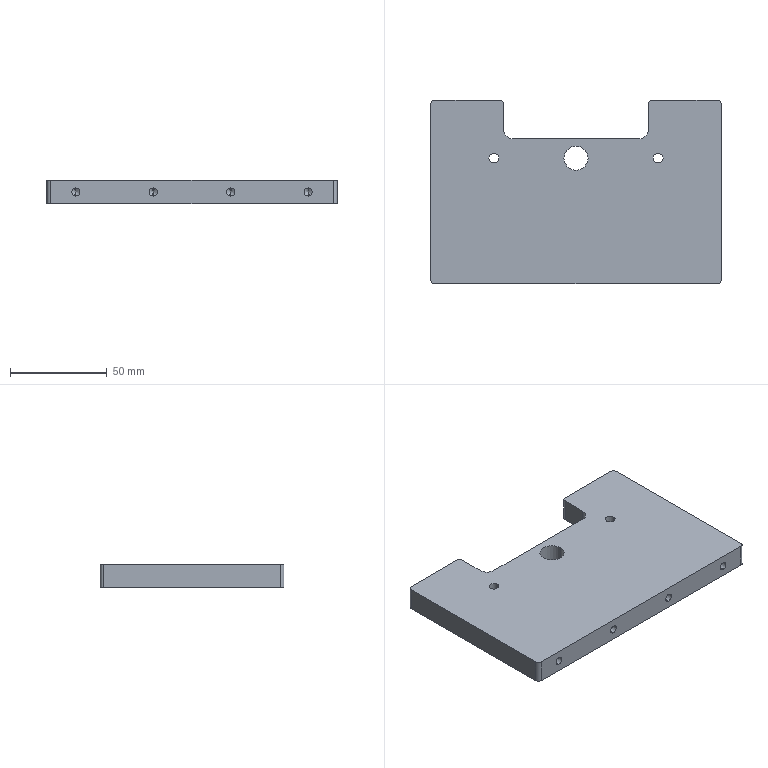Part | STEP file | 1 solid | 64 faces | box 150 x 95 x 12 mm | volume 149253 mm3 | cylinder 34 | cone 20 | plane 10 | commonest cylinder face diameters 4.2 x16 4 x10 5 x4 10 x2 12.5 x2